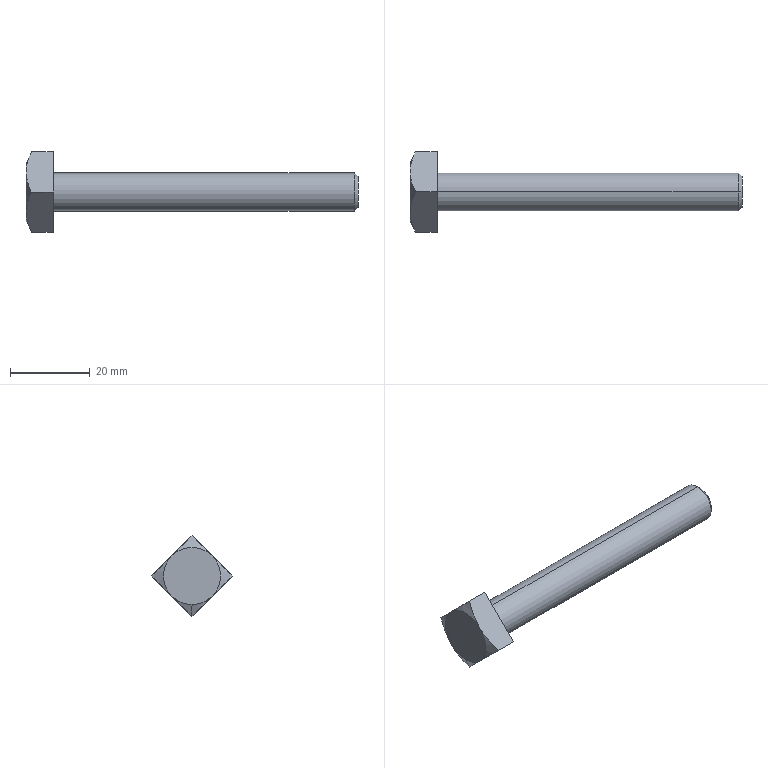Part | SolidWorks | features RevCut 2, Extrusion 1, Fillet 1, LPattern 1, Revolution 1 | 1 solid | 16 faces | box 83.007 x 20.188 x 20.188 mm | volume 6786 mm3 | cone 7 | plane 7 | cylinder 2 | commonest cylinder face diameters 9.525 x2
STEP:
#1=CARTESIAN_POINT('',(0.,0.,-0.281));
#2=VERTEX_POINT('',#1);
#3=CARTESIAN_POINT('',(0.,-0.1987,-0.1987));
#4=VERTEX_POINT('',#3);
#5=CARTESIAN_POINT('',(0.,0.,0.));
#6=DIRECTION('',(-1.,0.,0.));
#7=DIRECTION('',(0.,0.,-1.));
#8=AXIS2_PLACEMENT_3D('',#5,#6,#7);
#9=CIRCLE('',#8,0.281);
#10=EDGE_CURVE('',#2,#4,#9,.T.);
#11=ORIENTED_EDGE('',*,*,#10,.F.);
#12=CARTESIAN_POINT('',(0.05428,0.,-0.3974));
#13=VERTEX_POINT('',#12);
#14=CARTESIAN_POINT('',(0.,0.,-0.281));
#15=DIRECTION('',(0.4226,0.,-0.9063));
#16=VECTOR('',#15,39.37);
#17=LINE('',#14,#16);
#18=EDGE_CURVE('',#2,#13,#17,.T.);
#19=ORIENTED_EDGE('',*,*,#18,.T.);
#20=CARTESIAN_POINT('',(0.,-0.1987,-0.1987));
#21=CARTESIAN_POINT('',(0.,-0.1644,-0.233));
#22=CARTESIAN_POINT('',(0.006056,-0.1309,-0.2665));
#23=CARTESIAN_POINT('',(0.02576,-0.06485,-0.3325));
#24=CARTESIAN_POINT('',(0.0392,-0.03232,-0.3651));
#25=CARTESIAN_POINT('',(0.05428,0.,-0.3974));
#26=B_SPLINE_CURVE_WITH_KNOTS('',3,(#20,#21,#22,#23,#24,#25),.UNSPECIFIED.,.F.,.F.,(4,2,4),(0.00727,0.01092,0.01456),.UNSPECIFIED.);
#27=EDGE_CURVE('',#4,#13,#26,.T.);
#28=ORIENTED_EDGE('',*,*,#27,.F.);
#29=EDGE_LOOP('',(#11,#19,#28));
#30=FACE_OUTER_BOUND('',#29,.T.);
#31=CARTESIAN_POINT('',(0.,0.,0.));
#32=DIRECTION('',(1.,0.,0.));
#33=DIRECTION('',(0.,0.,-1.));
#34=AXIS2_PLACEMENT_3D('',#31,#32,#33);
#35=CONICAL_SURFACE('',#34,0.281,1.134);
#36=ADVANCED_FACE('',(#30),#35,.T.);
#37=CARTESIAN_POINT('',(3.231,0.,0.1875));
#38=VERTEX_POINT('',#37);
#39=CARTESIAN_POINT('',(3.231,0.,-0.1875));
#40=VERTEX_POINT('',#39);
#41=CARTESIAN_POINT('',(3.231,0.,0.));
#42=DIRECTION('',(-1.,0.,0.));
#43=DIRECTION('',(0.,0.,1.));
#44=AXIS2_PLACEMENT_3D('',#41,#42,#43);
#45=CIRCLE('',#44,0.1875);
#46=EDGE_CURVE('',#38,#40,#45,.T.);
#47=ORIENTED_EDGE('',*,*,#46,.T.);
#48=CARTESIAN_POINT('',(0.268,0.,-0.1875));
#49=VERTEX_POINT('',#48);
#50=CARTESIAN_POINT('',(0.,0.,-0.1875));
#51=DIRECTION('',(-1.,0.,0.));
#52=VECTOR('',#51,39.37);
#53=LINE('',#50,#52);
#54=EDGE_CURVE('',#40,#49,#53,.T.);
#55=ORIENTED_EDGE('',*,*,#54,.T.);
#56=CARTESIAN_POINT('',(0.268,0.,0.1875));
#57=VERTEX_POINT('',#56);
#58=CARTESIAN_POINT('',(0.268,0.,0.));
#59=DIRECTION('',(1.,0.,0.));
#60=DIRECTION('',(0.,0.,-1.));
#61=AXIS2_PLACEMENT_3D('',#58,#59,#60);
#62=CIRCLE('',#61,0.1875);
#63=EDGE_CURVE('',#49,#57,#62,.T.);
#64=ORIENTED_EDGE('',*,*,#63,.T.);
#65=CARTESIAN_POINT('',(0.,0.,0.1875));
#66=DIRECTION('',(-1.,0.,0.));
#67=VECTOR('',#66,39.37);
#68=LINE('',#65,#67);
#69=EDGE_CURVE('',#38,#57,#68,.T.);
#70=ORIENTED_EDGE('',*,*,#69,.F.);
#71=EDGE_LOOP('',(#47,#55,#64,#70));
#72=FACE_OUTER_BOUND('',#71,.T.);
#73=CARTESIAN_POINT('',(0.,0.,0.));
#74=DIRECTION('',(-1.,0.,0.));
#75=DIRECTION('',(0.,0.,1.));
#76=AXIS2_PLACEMENT_3D('',#73,#74,#75);
#77=CYLINDRICAL_SURFACE('',#76,0.1875);
#78=ADVANCED_FACE('',(#72),#77,.T.);
#79=CARTESIAN_POINT('',(3.268,0.,0.1502));
#80=VERTEX_POINT('',#79);
#81=CARTESIAN_POINT('',(3.268,0.,-0.1502));
#82=VERTEX_POINT('',#81);
#83=CARTESIAN_POINT('',(3.268,0.,0.));
#84=DIRECTION('',(-1.,0.,0.));
#85=DIRECTION('',(0.,0.,1.));
#86=AXIS2_PLACEMENT_3D('',#83,#84,#85);
#87=CIRCLE('',#86,0.1502);
#88=EDGE_CURVE('',#80,#82,#87,.T.);
#89=ORIENTED_EDGE('',*,*,#88,.T.);
#90=CARTESIAN_POINT('',(3.231,0.,-0.1875));
#91=DIRECTION('',(-0.7071,0.,-0.7071));
#92=VECTOR('',#91,39.37);
#93=LINE('',#90,#92);
#94=EDGE_CURVE('',#82,#40,#93,.T.);
#95=ORIENTED_EDGE('',*,*,#94,.T.);
#96=ORIENTED_EDGE('',*,*,#46,.F.);
#97=CARTESIAN_POINT('',(3.231,0.,0.1875));
#98=DIRECTION('',(-0.7071,0.,0.7071));
#99=VECTOR('',#98,39.37);
#100=LINE('',#97,#99);
#101=EDGE_CURVE('',#80,#38,#100,.T.);
#102=ORIENTED_EDGE('',*,*,#101,.F.);
#103=EDGE_LOOP('',(#89,#95,#96,#102));
#104=FACE_OUTER_BOUND('',#103,.T.);
#105=CARTESIAN_POINT('',(3.231,0.,0.));
#106=DIRECTION('',(-1.,0.,0.));
#107=DIRECTION('',(0.,0.,1.));
#108=AXIS2_PLACEMENT_3D('',#105,#106,#107);
#109=CONICAL_SURFACE('',#108,0.1875,0.7854);
#110=ADVANCED_FACE('',(#104),#109,.T.);
#111=CARTESIAN_POINT('',(0.05428,0.3974,0.));
#112=VERTEX_POINT('',#111);
#113=CARTESIAN_POINT('',(0.,0.1987,-0.1987));
#114=VERTEX_POINT('',#113);
#115=CARTESIAN_POINT('',(0.05428,0.3974,0.));
#116=CARTESIAN_POINT('',(0.03923,0.3651,-0.03227));
#117=CARTESIAN_POINT('',(0.02579,0.3326,-0.06477));
#118=CARTESIAN_POINT('',(0.011,0.2831,-0.1143));
#119=CARTESIAN_POINT('',(0.006998,0.2665,-0.1309));
#120=CARTESIAN_POINT('',(0.002866,0.2413,-0.1561));
#121=CARTESIAN_POINT('',(0.001802,0.2328,-0.1646));
#122=CARTESIAN_POINT('',(0.0003684,0.2158,-0.1816));
#123=CARTESIAN_POINT('',(0.,0.2072,-0.1901));
#124=CARTESIAN_POINT('',(0.,0.1987,-0.1987));
#125=B_SPLINE_CURVE_WITH_KNOTS('',3,(#115,#116,#117,#118,#119,#120,#121,#122,#123,#124),.UNSPECIFIED.,.F.,.F.,(4,2,2,2,4),(0.000000296,0.003635,0.005453,0.006361,0.00727),.UNSPECIFIED.);
#126=EDGE_CURVE('',#112,#114,#125,.T.);
#127=ORIENTED_EDGE('',*,*,#126,.F.);
#128=CARTESIAN_POINT('',(0.268,0.3974,0.));
#129=VERTEX_POINT('',#128);
#130=CARTESIAN_POINT('',(0.268,0.3974,0.));
#131=DIRECTION('',(-1.,0.,0.));
#132=VECTOR('',#131,39.37);
#133=LINE('',#130,#132);
#134=EDGE_CURVE('',#129,#112,#133,.T.);
#135=ORIENTED_EDGE('',*,*,#134,.F.);
#136=CARTESIAN_POINT('',(0.268,0.,-0.3974));
#137=VERTEX_POINT('',#136);
#138=CARTESIAN_POINT('',(0.268,0.,-0.3974));
#139=DIRECTION('',(0.,0.7071,0.7071));
#140=VECTOR('',#139,39.37);
#141=LINE('',#138,#140);
#142=EDGE_CURVE('',#137,#129,#141,.T.);
#143=ORIENTED_EDGE('',*,*,#142,.F.);
#144=CARTESIAN_POINT('',(0.268,0.,-0.3974));
#145=DIRECTION('',(-1.,0.,0.));
#146=VECTOR('',#145,39.37);
#147=LINE('',#144,#146);
#148=EDGE_CURVE('',#137,#13,#147,.T.);
#149=ORIENTED_EDGE('',*,*,#148,.T.);
#150=CARTESIAN_POINT('',(0.,0.1987,-0.1987));
#151=CARTESIAN_POINT('',(0.,0.1644,-0.233));
#152=CARTESIAN_POINT('',(0.006056,0.1309,-0.2665));
#153=CARTESIAN_POINT('',(0.02576,0.06485,-0.3325));
#154=CARTESIAN_POINT('',(0.0392,0.03232,-0.3651));
#155=CARTESIAN_POINT('',(0.05428,0.,-0.3974));
#156=B_SPLINE_CURVE_WITH_KNOTS('',3,(#150,#151,#152,#153,#154,#155),.UNSPECIFIED.,.F.,.F.,(4,2,4),(0.00727,0.01092,0.01456),.UNSPECIFIED.);
#157=EDGE_CURVE('',#114,#13,#156,.T.);
#158=ORIENTED_EDGE('',*,*,#157,.F.);
#159=EDGE_LOOP('',(#127,#135,#143,#149,#158));
#160=FACE_OUTER_BOUND('',#159,.T.);
#161=CARTESIAN_POINT('',(0.268,0.,-0.3974));
#162=DIRECTION('',(0.,-0.7071,0.7071));
#163=DIRECTION('',(0.,-0.7071,-0.7071));
#164=AXIS2_PLACEMENT_3D('',#161,#162,#163);
#165=PLANE('',#164);
#166=ADVANCED_FACE('',(#160),#165,.F.);
#167=ORIENTED_EDGE('',*,*,#134,.T.);
#168=CARTESIAN_POINT('',(0.,0.1987,0.1987));
#169=VERTEX_POINT('',#168);
#170=CARTESIAN_POINT('',(0.05428,0.3974,0.));
#171=CARTESIAN_POINT('',(0.03923,0.3651,0.03227));
#172=CARTESIAN_POINT('',(0.02579,0.3326,0.06477));
#173=CARTESIAN_POINT('',(0.011,0.2831,0.1143));
#174=CARTESIAN_POINT('',(0.006998,0.2665,0.1309));
#175=CARTESIAN_POINT('',(0.002866,0.2413,0.1561));
#176=CARTESIAN_POINT('',(0.001802,0.2328,0.1646));
#177=CARTESIAN_POINT('',(0.0003684,0.2158,0.1816));
#178=CARTESIAN_POINT('',(0.,0.2072,0.1901));
#179=CARTESIAN_POINT('',(0.,0.1987,0.1987));
#180=B_SPLINE_CURVE_WITH_KNOTS('',3,(#170,#171,#172,#173,#174,#175,#176,#177,#178,#179),.UNSPECIFIED.,.F.,.F.,(4,2,2,2,4),(0.000000296,0.003635,0.005453,0.006361,0.00727),.UNSPECIFIED.);
#181=EDGE_CURVE('',#112,#169,#180,.T.);
#182=ORIENTED_EDGE('',*,*,#181,.T.);
#183=CARTESIAN_POINT('',(0.05428,0.,0.3974));
#184=VERTEX_POINT('',#183);
#185=CARTESIAN_POINT('',(0.,0.1987,0.1987));
#186=CARTESIAN_POINT('',(0.,0.1644,0.233));
#187=CARTESIAN_POINT('',(0.006056,0.1309,0.2665));
#188=CARTESIAN_POINT('',(0.02576,0.06485,0.3325));
#189=CARTESIAN_POINT('',(0.0392,0.03232,0.3651));
#190=CARTESIAN_POINT('',(0.05428,0.,0.3974));
#191=B_SPLINE_CURVE_WITH_KNOTS('',3,(#185,#186,#187,#188,#189,#190),.UNSPECIFIED.,.F.,.F.,(4,2,4),(0.00727,0.01092,0.01456),.UNSPECIFIED.);
#192=EDGE_CURVE('',#169,#184,#191,.T.);
#193=ORIENTED_EDGE('',*,*,#192,.T.);
#194=CARTESIAN_POINT('',(0.268,0.,0.3974));
#195=VERTEX_POINT('',#194);
#196=CARTESIAN_POINT('',(0.268,0.,0.3974));
#197=DIRECTION('',(-1.,0.,0.));
#198=VECTOR('',#197,39.37);
#199=LINE('',#196,#198);
#200=EDGE_CURVE('',#195,#184,#199,.T.);
#201=ORIENTED_EDGE('',*,*,#200,.F.);
#202=CARTESIAN_POINT('',(0.268,0.,0.3974));
#203=DIRECTION('',(0.,0.7071,-0.7071));
#204=VECTOR('',#203,39.37);
#205=LINE('',#202,#204);
#206=EDGE_CURVE('',#195,#129,#205,.T.);
#207=ORIENTED_EDGE('',*,*,#206,.T.);
#208=EDGE_LOOP('',(#167,#182,#193,#201,#207));
#209=FACE_OUTER_BOUND('',#208,.T.);
#210=CARTESIAN_POINT('',(0.268,0.,0.3974));
#211=DIRECTION('',(0.,0.7071,0.7071));
#212=DIRECTION('',(0.,-0.7071,0.7071));
#213=AXIS2_PLACEMENT_3D('',#210,#211,#212);
#214=PLANE('',#213);
#215=ADVANCED_FACE('',(#209),#214,.T.);
#216=CARTESIAN_POINT('',(0.05428,-0.3974,0.));
#217=VERTEX_POINT('',#216);
#218=CARTESIAN_POINT('',(0.,-0.1987,0.1987));
#219=VERTEX_POINT('',#218);
#220=CARTESIAN_POINT('',(0.05428,-0.3974,0.));
#221=CARTESIAN_POINT('',(0.03923,-0.3651,0.03227));
#222=CARTESIAN_POINT('',(0.02579,-0.3326,0.06477));
#223=CARTESIAN_POINT('',(0.011,-0.2831,0.1143));
#224=CARTESIAN_POINT('',(0.006998,-0.2665,0.1309));
#225=CARTESIAN_POINT('',(0.002866,-0.2413,0.1561));
#226=CARTESIAN_POINT('',(0.001802,-0.2328,0.1646));
#227=CARTESIAN_POINT('',(0.0003684,-0.2158,0.1816));
#228=CARTESIAN_POINT('',(0.,-0.2072,0.1901));
#229=CARTESIAN_POINT('',(0.,-0.1987,0.1987));
#230=B_SPLINE_CURVE_WITH_KNOTS('',3,(#220,#221,#222,#223,#224,#225,#226,#227,#228,#229),.UNSPECIFIED.,.F.,.F.,(4,2,2,2,4),(0.000000296,0.003635,0.005453,0.006361,0.00727),.UNSPECIFIED.);
#231=EDGE_CURVE('',#217,#219,#230,.T.);
#232=ORIENTED_EDGE('',*,*,#231,.F.);
#233=CARTESIAN_POINT('',(0.268,-0.3974,0.));
#234=VERTEX_POINT('',#233);
#235=CARTESIAN_POINT('',(0.268,-0.3974,0.));
#236=DIRECTION('',(-1.,0.,0.));
#237=VECTOR('',#236,39.37);
#238=LINE('',#235,#237);
#239=EDGE_CURVE('',#234,#217,#238,.T.);
#240=ORIENTED_EDGE('',*,*,#239,.F.);
#241=CARTESIAN_POINT('',(0.268,0.,0.3974));
#242=DIRECTION('',(0.,-0.7071,-0.7071));
#243=VECTOR('',#242,39.37);
#244=LINE('',#241,#243);
#245=EDGE_CURVE('',#195,#234,#244,.T.);
#246=ORIENTED_EDGE('',*,*,#245,.F.);
#247=ORIENTED_EDGE('',*,*,#200,.T.);
#248=CARTESIAN_POINT('',(0.,-0.1987,0.1987));
#249=CARTESIAN_POINT('',(0.,-0.1644,0.233));
#250=CARTESIAN_POINT('',(0.006056,-0.1309,0.2665));
#251=CARTESIAN_POINT('',(0.02576,-0.06485,0.3325));
#252=CARTESIAN_POINT('',(0.0392,-0.03232,0.3651));
#253=CARTESIAN_POINT('',(0.05428,0.,0.3974));
#254=B_SPLINE_CURVE_WITH_KNOTS('',3,(#248,#249,#250,#251,#252,#253),.UNSPECIFIED.,.F.,.F.,(4,2,4),(0.00727,0.01092,0.01456),.UNSPECIFIED.);
#255=EDGE_CURVE('',#219,#184,#254,.T.);
#256=ORIENTED_EDGE('',*,*,#255,.F.);
#257=EDGE_LOOP('',(#232,#240,#246,#247,#256));
#258=FACE_OUTER_BOUND('',#257,.T.);
#259=CARTESIAN_POINT('',(0.268,0.,0.3974));
#260=DIRECTION('',(0.,0.7071,-0.7071));
#261=DIRECTION('',(0.,0.7071,0.7071));
#262=AXIS2_PLACEMENT_3D('',#259,#260,#261);
#263=PLANE('',#262);
#264=ADVANCED_FACE('',(#258),#263,.F.);
#265=ORIENTED_EDGE('',*,*,#239,.T.);
#266=CARTESIAN_POINT('',(0.05428,-0.3974,0.));
#267=CARTESIAN_POINT('',(0.03923,-0.3651,-0.03227));
#268=CARTESIAN_POINT('',(0.02579,-0.3326,-0.06477));
#269=CARTESIAN_POINT('',(0.011,-0.2831,-0.1143));
#270=CARTESIAN_POINT('',(0.006998,-0.2665,-0.1309));
#271=CARTESIAN_POINT('',(0.002866,-0.2413,-0.1561));
#272=CARTESIAN_POINT('',(0.001802,-0.2328,-0.1646));
#273=CARTESIAN_POINT('',(0.0003684,-0.2158,-0.1816));
#274=CARTESIAN_POINT('',(0.,-0.2072,-0.1901));
#275=CARTESIAN_POINT('',(0.,-0.1987,-0.1987));
#276=B_SPLINE_CURVE_WITH_KNOTS('',3,(#266,#267,#268,#269,#270,#271,#272,#273,#274,#275),.UNSPECIFIED.,.F.,.F.,(4,2,2,2,4),(0.000000296,0.003635,0.005453,0.006361,0.00727),.UNSPECIFIED.);
#277=EDGE_CURVE('',#217,#4,#276,.T.);
#278=ORIENTED_EDGE('',*,*,#277,.T.);
#279=ORIENTED_EDGE('',*,*,#27,.T.);
#280=ORIENTED_EDGE('',*,*,#148,.F.);
#281=CARTESIAN_POINT('',(0.268,0.,-0.3974));
#282=DIRECTION('',(0.,-0.7071,0.7071));
#283=VECTOR('',#282,39.37);
#284=LINE('',#281,#283);
#285=EDGE_CURVE('',#137,#234,#284,.T.);
#286=ORIENTED_EDGE('',*,*,#285,.T.);
#287=EDGE_LOOP('',(#265,#278,#279,#280,#286));
#288=FACE_OUTER_BOUND('',#287,.T.);
#289=CARTESIAN_POINT('',(0.268,0.,-0.3974));
#290=DIRECTION('',(0.,-0.7071,-0.7071));
#291=DIRECTION('',(0.,0.7071,-0.7071));
#292=AXIS2_PLACEMENT_3D('',#289,#290,#291);
#293=PLANE('',#292);
#294=ADVANCED_FACE('',(#288),#293,.T.);
#295=CARTESIAN_POINT('',(0.268,0.,0.));
#296=DIRECTION('',(1.,0.,0.));
#297=DIRECTION('',(0.,0.,-1.));
#298=AXIS2_PLACEMENT_3D('',#295,#296,#297);
#299=CIRCLE('',#298,0.1875);
#300=EDGE_CURVE('',#57,#49,#299,.T.);
#301=ORIENTED_EDGE('',*,*,#300,.F.);
#302=ORIENTED_EDGE('',*,*,#63,.F.);
#303=EDGE_LOOP('',(#301,#302));
#304=FACE_BOUND('',#303,.T.);
#305=ORIENTED_EDGE('',*,*,#142,.T.);
#306=ORIENTED_EDGE('',*,*,#206,.F.);
#307=ORIENTED_EDGE('',*,*,#245,.T.);
#308=ORIENTED_EDGE('',*,*,#285,.F.);
#309=EDGE_LOOP('',(#305,#306,#307,#308));
#310=FACE_OUTER_BOUND('',#309,.T.);
#311=CARTESIAN_POINT('',(0.268,0.,-0.3974));
#312=DIRECTION('',(1.,0.,0.));
#313=DIRECTION('',(0.,0.,-1.));
#314=AXIS2_PLACEMENT_3D('',#311,#312,#313);
#315=PLANE('',#314);
#316=ADVANCED_FACE('',(#304,#310),#315,.T.);
#317=ORIENTED_EDGE('',*,*,#88,.F.);
#318=CARTESIAN_POINT('',(3.268,0.,0.));
#319=DIRECTION('',(-1.,0.,0.));
#320=DIRECTION('',(0.,0.,1.));
#321=AXIS2_PLACEMENT_3D('',#318,#319,#320);
#322=CIRCLE('',#321,0.1502);
#323=EDGE_CURVE('',#82,#80,#322,.T.);
#324=ORIENTED_EDGE('',*,*,#323,.F.);
#325=EDGE_LOOP('',(#317,#324));
#326=FACE_OUTER_BOUND('',#325,.T.);
#327=CARTESIAN_POINT('',(3.268,0.1502,0.));
#328=DIRECTION('',(1.,0.,0.));
#329=DIRECTION('',(0.,0.,-1.));
#330=AXIS2_PLACEMENT_3D('',#327,#328,#329);
#331=PLANE('',#330);
#332=ADVANCED_FACE('',(#326),#331,.T.);
#333=ORIENTED_EDGE('',*,*,#94,.F.);
#334=ORIENTED_EDGE('',*,*,#323,.T.);
#335=ORIENTED_EDGE('',*,*,#101,.T.);
#336=CARTESIAN_POINT('',(3.231,0.,0.));
#337=DIRECTION('',(-1.,0.,0.));
#338=DIRECTION('',(0.,0.,1.));
#339=AXIS2_PLACEMENT_3D('',#336,#337,#338);
#340=CIRCLE('',#339,0.1875);
#341=EDGE_CURVE('',#40,#38,#340,.T.);
#342=ORIENTED_EDGE('',*,*,#341,.F.);
#343=EDGE_LOOP('',(#333,#334,#335,#342));
#344=FACE_OUTER_BOUND('',#343,.T.);
#345=CARTESIAN_POINT('',(3.231,0.,0.));
#346=DIRECTION('',(-1.,0.,0.));
#347=DIRECTION('',(0.,0.,1.));
#348=AXIS2_PLACEMENT_3D('',#345,#346,#347);
#349=CONICAL_SURFACE('',#348,0.1875,0.7854);
#350=ADVANCED_FACE('',(#344),#349,.T.);
#351=ORIENTED_EDGE('',*,*,#54,.F.);
#352=ORIENTED_EDGE('',*,*,#341,.T.);
#353=ORIENTED_EDGE('',*,*,#69,.T.);
#354=ORIENTED_EDGE('',*,*,#300,.T.);
#355=EDGE_LOOP('',(#351,#352,#353,#354));
#356=FACE_OUTER_BOUND('',#355,.T.);
#357=CARTESIAN_POINT('',(0.,0.,0.));
#358=DIRECTION('',(-1.,0.,0.));
#359=DIRECTION('',(0.,0.,1.));
#360=AXIS2_PLACEMENT_3D('',#357,#358,#359);
#361=CYLINDRICAL_SURFACE('',#360,0.1875);
#362=ADVANCED_FACE('',(#356),#361,.T.);
#363=ORIENTED_EDGE('',*,*,#18,.F.);
#364=CARTESIAN_POINT('',(0.,0.,0.));
#365=DIRECTION('',(-1.,0.,0.));
#366=DIRECTION('',(0.,0.,-1.));
#367=AXIS2_PLACEMENT_3D('',#364,#365,#366);
#368=CIRCLE('',#367,0.281);
#369=EDGE_CURVE('',#114,#2,#368,.T.);
#370=ORIENTED_EDGE('',*,*,#369,.F.);
#371=ORIENTED_EDGE('',*,*,#157,.T.);
#372=EDGE_LOOP('',(#363,#370,#371));
#373=FACE_OUTER_BOUND('',#372,.T.);
#374=CARTESIAN_POINT('',(0.,0.,0.));
#375=DIRECTION('',(1.,0.,0.));
#376=DIRECTION('',(0.,0.,-1.));
#377=AXIS2_PLACEMENT_3D('',#374,#375,#376);
#378=CONICAL_SURFACE('',#377,0.281,1.134);
#379=ADVANCED_FACE('',(#373),#378,.T.);
#380=ORIENTED_EDGE('',*,*,#126,.T.);
#381=CARTESIAN_POINT('',(0.,0.,0.));
#382=DIRECTION('',(-1.,0.,0.));
#383=DIRECTION('',(0.,0.,1.));
#384=AXIS2_PLACEMENT_3D('',#381,#382,#383);
#385=CIRCLE('',#384,0.281);
#386=EDGE_CURVE('',#169,#114,#385,.T.);
#387=ORIENTED_EDGE('',*,*,#386,.F.);
#388=ORIENTED_EDGE('',*,*,#181,.F.);
#389=EDGE_LOOP('',(#380,#387,#388));
#390=FACE_OUTER_BOUND('',#389,.T.);
#391=CARTESIAN_POINT('',(0.,0.,0.));
#392=DIRECTION('',(1.,0.,0.));
#393=DIRECTION('',(0.,0.,-1.));
#394=AXIS2_PLACEMENT_3D('',#391,#392,#393);
#395=CONICAL_SURFACE('',#394,0.281,1.134);
#396=ADVANCED_FACE('',(#390),#395,.T.);
#397=CARTESIAN_POINT('',(0.,0.,0.));
#398=DIRECTION('',(-1.,0.,0.));
#399=DIRECTION('',(0.,0.,-1.));
#400=AXIS2_PLACEMENT_3D('',#397,#398,#399);
#401=CIRCLE('',#400,0.281);
#402=EDGE_CURVE('',#219,#169,#401,.T.);
#403=ORIENTED_EDGE('',*,*,#402,.F.);
#404=ORIENTED_EDGE('',*,*,#255,.T.);
#405=ORIENTED_EDGE('',*,*,#192,.F.);
#406=EDGE_LOOP('',(#403,#404,#405));
#407=FACE_OUTER_BOUND('',#406,.T.);
#408=CARTESIAN_POINT('',(0.,0.,0.));
#409=DIRECTION('',(1.,0.,0.));
#410=DIRECTION('',(0.,0.,-1.));
#411=AXIS2_PLACEMENT_3D('',#408,#409,#410);
#412=CONICAL_SURFACE('',#411,0.281,1.134);
#413=ADVANCED_FACE('',(#407),#412,.T.);
#414=ORIENTED_EDGE('',*,*,#231,.T.);
#415=CARTESIAN_POINT('',(0.,0.,0.));
#416=DIRECTION('',(-1.,0.,0.));
#417=DIRECTION('',(0.,0.,-1.));
#418=AXIS2_PLACEMENT_3D('',#415,#416,#417);
#419=CIRCLE('',#418,0.281);
#420=EDGE_CURVE('',#4,#219,#419,.T.);
#421=ORIENTED_EDGE('',*,*,#420,.F.);
#422=ORIENTED_EDGE('',*,*,#277,.F.);
#423=EDGE_LOOP('',(#414,#421,#422));
#424=FACE_OUTER_BOUND('',#423,.T.);
#425=CARTESIAN_POINT('',(0.,0.,0.));
#426=DIRECTION('',(1.,0.,0.));
#427=DIRECTION('',(0.,0.,-1.));
#428=AXIS2_PLACEMENT_3D('',#425,#426,#427);
#429=CONICAL_SURFACE('',#428,0.281,1.134);
#430=ADVANCED_FACE('',(#424),#429,.T.);
#431=ORIENTED_EDGE('',*,*,#369,.T.);
#432=ORIENTED_EDGE('',*,*,#10,.T.);
#433=ORIENTED_EDGE('',*,*,#420,.T.);
#434=ORIENTED_EDGE('',*,*,#402,.T.);
#435=ORIENTED_EDGE('',*,*,#386,.T.);
#436=EDGE_LOOP('',(#431,#432,#433,#434,#435));
#437=FACE_OUTER_BOUND('',#436,.T.);
#438=CARTESIAN_POINT('',(0.,0.,-0.3974));
#439=DIRECTION('',(1.,0.,0.));
#440=DIRECTION('',(0.,0.,-1.));
#441=AXIS2_PLACEMENT_3D('',#438,#439,#440);
#442=PLANE('',#441);
#443=ADVANCED_FACE('',(#437),#442,.F.);
#444=CLOSED_SHELL('',(#36,#78,#110,#166,#215,#264,#294,#316,#332,#350,#362,#379,#396,#413,#430,#443));
#445=MANIFOLD_SOLID_BREP('',#444);
#446=CARTESIAN_POINT('',(0.,0.,0.));
#447=DIRECTION('',(0.,0.,1.));
#448=DIRECTION('',(1.,0.,0.));
#449=AXIS2_PLACEMENT_3D('',#446,#447,#448);
#450=(LENGTH_UNIT()NAMED_UNIT(*)SI_UNIT($,.METRE.));
#451=LENGTH_MEASURE_WITH_UNIT(LENGTH_MEASURE(0.0254),#450);
#452=DIMENSIONAL_EXPONENTS(1.,0.,0.,0.,0.,0.,0.);
#453=(CONVERSION_BASED_UNIT('INCH',#451)LENGTH_UNIT()NAMED_UNIT(#452));
#454=UNCERTAINTY_MEASURE_WITH_UNIT(LENGTH_MEASURE(0.00001),#453,'','');
#455=(NAMED_UNIT(*)PLANE_ANGLE_UNIT()SI_UNIT($,.RADIAN.));
#456=(NAMED_UNIT(*)SI_UNIT($,.STERADIAN.)SOLID_ANGLE_UNIT());
#457=(GEOMETRIC_REPRESENTATION_CONTEXT(3)GLOBAL_UNCERTAINTY_ASSIGNED_CONTEXT((#454))GLOBAL_UNIT_ASSIGNED_CONTEXT((#453,#455,#456))REPRESENTATION_CONTEXT('',''));
#458=ADVANCED_BREP_SHAPE_REPRESENTATION('',(#445,#449),#457);